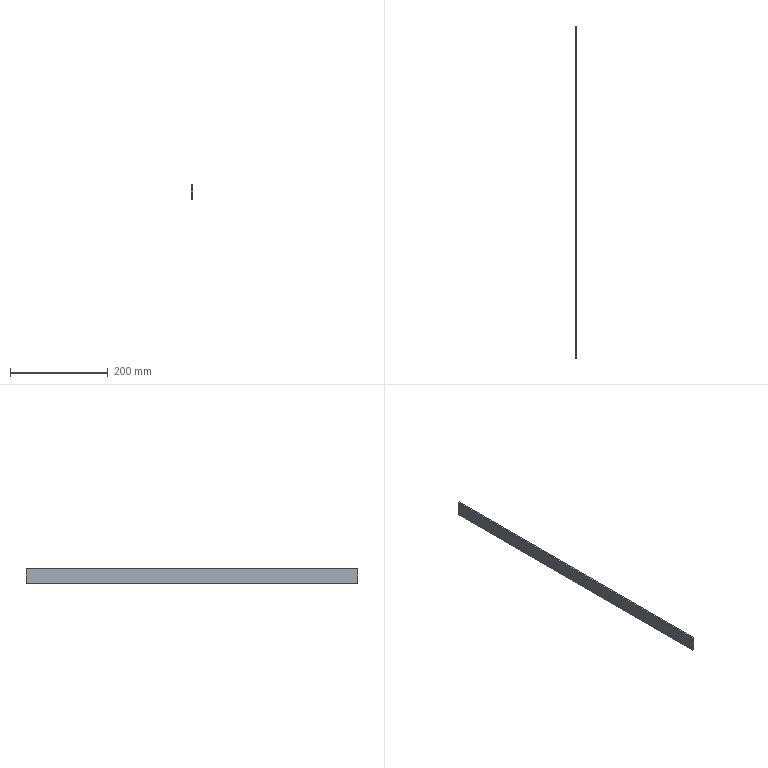Part | SolidWorks | 1 solid | 6 faces | box 3 x 680 x 30 mm | volume 61200 mm3 | plane 6
STEP:
#1=CARTESIAN_POINT('',(0.,340.,15.));
#2=VERTEX_POINT('',#1);
#3=CARTESIAN_POINT('',(0.,-340.,15.));
#4=VERTEX_POINT('',#3);
#5=CARTESIAN_POINT('',(0.,-340.,15.));
#6=DIRECTION('',(0.,-1.,0.));
#7=VECTOR('',#6,1000.);
#8=LINE('',#5,#7);
#9=EDGE_CURVE('',#2,#4,#8,.T.);
#10=ORIENTED_EDGE('',*,*,#9,.F.);
#11=CARTESIAN_POINT('',(-3.,340.,15.));
#12=VERTEX_POINT('',#11);
#13=CARTESIAN_POINT('',(-3.,340.,15.));
#14=DIRECTION('',(1.,0.,0.));
#15=VECTOR('',#14,1000.);
#16=LINE('',#13,#15);
#17=EDGE_CURVE('',#12,#2,#16,.T.);
#18=ORIENTED_EDGE('',*,*,#17,.F.);
#19=CARTESIAN_POINT('',(-3.,-340.,15.));
#20=VERTEX_POINT('',#19);
#21=CARTESIAN_POINT('',(-3.,-340.,15.));
#22=DIRECTION('',(0.,-1.,0.));
#23=VECTOR('',#22,1000.);
#24=LINE('',#21,#23);
#25=EDGE_CURVE('',#12,#20,#24,.T.);
#26=ORIENTED_EDGE('',*,*,#25,.T.);
#27=CARTESIAN_POINT('',(-3.,-340.,15.));
#28=DIRECTION('',(1.,0.,0.));
#29=VECTOR('',#28,1000.);
#30=LINE('',#27,#29);
#31=EDGE_CURVE('',#20,#4,#30,.T.);
#32=ORIENTED_EDGE('',*,*,#31,.T.);
#33=EDGE_LOOP('',(#10,#18,#26,#32));
#34=FACE_OUTER_BOUND('',#33,.T.);
#35=CARTESIAN_POINT('',(-3.,-340.,15.));
#36=DIRECTION('',(0.,0.,1.));
#37=DIRECTION('',(1.,0.,0.));
#38=AXIS2_PLACEMENT_3D('',#35,#36,#37);
#39=PLANE('',#38);
#40=ADVANCED_FACE('',(#34),#39,.T.);
#41=CARTESIAN_POINT('',(0.,340.,-15.));
#42=VERTEX_POINT('',#41);
#43=CARTESIAN_POINT('',(0.,340.,-15.));
#44=DIRECTION('',(0.,0.,1.));
#45=VECTOR('',#44,1000.);
#46=LINE('',#43,#45);
#47=EDGE_CURVE('',#42,#2,#46,.T.);
#48=ORIENTED_EDGE('',*,*,#47,.F.);
#49=CARTESIAN_POINT('',(-3.,340.,-15.));
#50=VERTEX_POINT('',#49);
#51=CARTESIAN_POINT('',(-3.,340.,-15.));
#52=DIRECTION('',(1.,0.,0.));
#53=VECTOR('',#52,1000.);
#54=LINE('',#51,#53);
#55=EDGE_CURVE('',#50,#42,#54,.T.);
#56=ORIENTED_EDGE('',*,*,#55,.F.);
#57=CARTESIAN_POINT('',(-3.,340.,-15.));
#58=DIRECTION('',(0.,0.,1.));
#59=VECTOR('',#58,1000.);
#60=LINE('',#57,#59);
#61=EDGE_CURVE('',#50,#12,#60,.T.);
#62=ORIENTED_EDGE('',*,*,#61,.T.);
#63=ORIENTED_EDGE('',*,*,#17,.T.);
#64=EDGE_LOOP('',(#48,#56,#62,#63));
#65=FACE_OUTER_BOUND('',#64,.T.);
#66=CARTESIAN_POINT('',(-3.,340.,-15.));
#67=DIRECTION('',(0.,1.,0.));
#68=DIRECTION('',(0.,0.,1.));
#69=AXIS2_PLACEMENT_3D('',#66,#67,#68);
#70=PLANE('',#69);
#71=ADVANCED_FACE('',(#65),#70,.T.);
#72=CARTESIAN_POINT('',(0.,-340.,-15.));
#73=VERTEX_POINT('',#72);
#74=CARTESIAN_POINT('',(0.,-340.,-15.));
#75=DIRECTION('',(0.,1.,0.));
#76=VECTOR('',#75,1000.);
#77=LINE('',#74,#76);
#78=EDGE_CURVE('',#73,#42,#77,.T.);
#79=ORIENTED_EDGE('',*,*,#78,.F.);
#80=CARTESIAN_POINT('',(-3.,-340.,-15.));
#81=VERTEX_POINT('',#80);
#82=CARTESIAN_POINT('',(-3.,-340.,-15.));
#83=DIRECTION('',(1.,0.,0.));
#84=VECTOR('',#83,1000.);
#85=LINE('',#82,#84);
#86=EDGE_CURVE('',#81,#73,#85,.T.);
#87=ORIENTED_EDGE('',*,*,#86,.F.);
#88=CARTESIAN_POINT('',(-3.,-340.,-15.));
#89=DIRECTION('',(0.,1.,0.));
#90=VECTOR('',#89,1000.);
#91=LINE('',#88,#90);
#92=EDGE_CURVE('',#81,#50,#91,.T.);
#93=ORIENTED_EDGE('',*,*,#92,.T.);
#94=ORIENTED_EDGE('',*,*,#55,.T.);
#95=EDGE_LOOP('',(#79,#87,#93,#94));
#96=FACE_OUTER_BOUND('',#95,.T.);
#97=CARTESIAN_POINT('',(-3.,-340.,-15.));
#98=DIRECTION('',(0.,0.,-1.));
#99=DIRECTION('',(-1.,0.,0.));
#100=AXIS2_PLACEMENT_3D('',#97,#98,#99);
#101=PLANE('',#100);
#102=ADVANCED_FACE('',(#96),#101,.T.);
#103=CARTESIAN_POINT('',(0.,-340.,-15.));
#104=DIRECTION('',(0.,0.,-1.));
#105=VECTOR('',#104,1000.);
#106=LINE('',#103,#105);
#107=EDGE_CURVE('',#4,#73,#106,.T.);
#108=ORIENTED_EDGE('',*,*,#107,.F.);
#109=ORIENTED_EDGE('',*,*,#31,.F.);
#110=CARTESIAN_POINT('',(-3.,-340.,-15.));
#111=DIRECTION('',(0.,0.,-1.));
#112=VECTOR('',#111,1000.);
#113=LINE('',#110,#112);
#114=EDGE_CURVE('',#20,#81,#113,.T.);
#115=ORIENTED_EDGE('',*,*,#114,.T.);
#116=ORIENTED_EDGE('',*,*,#86,.T.);
#117=EDGE_LOOP('',(#108,#109,#115,#116));
#118=FACE_OUTER_BOUND('',#117,.T.);
#119=CARTESIAN_POINT('',(-3.,-340.,-15.));
#120=DIRECTION('',(0.,-1.,0.));
#121=DIRECTION('',(0.,0.,-1.));
#122=AXIS2_PLACEMENT_3D('',#119,#120,#121);
#123=PLANE('',#122);
#124=ADVANCED_FACE('',(#118),#123,.T.);
#125=ORIENTED_EDGE('',*,*,#25,.F.);
#126=ORIENTED_EDGE('',*,*,#61,.F.);
#127=ORIENTED_EDGE('',*,*,#92,.F.);
#128=ORIENTED_EDGE('',*,*,#114,.F.);
#129=EDGE_LOOP('',(#125,#126,#127,#128));
#130=FACE_OUTER_BOUND('',#129,.T.);
#131=CARTESIAN_POINT('',(-3.,0.,0.));
#132=DIRECTION('',(1.,0.,0.));
#133=DIRECTION('',(0.,0.,-1.));
#134=AXIS2_PLACEMENT_3D('',#131,#132,#133);
#135=PLANE('',#134);
#136=ADVANCED_FACE('',(#130),#135,.F.);
#137=ORIENTED_EDGE('',*,*,#9,.T.);
#138=ORIENTED_EDGE('',*,*,#107,.T.);
#139=ORIENTED_EDGE('',*,*,#78,.T.);
#140=ORIENTED_EDGE('',*,*,#47,.T.);
#141=EDGE_LOOP('',(#137,#138,#139,#140));
#142=FACE_OUTER_BOUND('',#141,.T.);
#143=CARTESIAN_POINT('',(0.,0.,0.));
#144=DIRECTION('',(1.,0.,0.));
#145=DIRECTION('',(0.,0.,-1.));
#146=AXIS2_PLACEMENT_3D('',#143,#144,#145);
#147=PLANE('',#146);
#148=ADVANCED_FACE('',(#142),#147,.T.);
#149=CLOSED_SHELL('',(#40,#71,#102,#124,#136,#148));
#150=MANIFOLD_SOLID_BREP('',#149);
#151=CARTESIAN_POINT('',(0.,0.,0.));
#152=DIRECTION('',(0.,0.,1.));
#153=DIRECTION('',(1.,0.,0.));
#154=AXIS2_PLACEMENT_3D('',#151,#152,#153);
#155=(LENGTH_UNIT()NAMED_UNIT(*)SI_UNIT(.MILLI.,.METRE.));
#156=UNCERTAINTY_MEASURE_WITH_UNIT(LENGTH_MEASURE(0.00001),#155,'','');
#157=(NAMED_UNIT(*)PLANE_ANGLE_UNIT()SI_UNIT($,.RADIAN.));
#158=(NAMED_UNIT(*)SI_UNIT($,.STERADIAN.)SOLID_ANGLE_UNIT());
#159=(GEOMETRIC_REPRESENTATION_CONTEXT(3)GLOBAL_UNCERTAINTY_ASSIGNED_CONTEXT((#156))GLOBAL_UNIT_ASSIGNED_CONTEXT((#155,#157,#158))REPRESENTATION_CONTEXT('',''));
#160=ADVANCED_BREP_SHAPE_REPRESENTATION('',(#150,#154),#159);